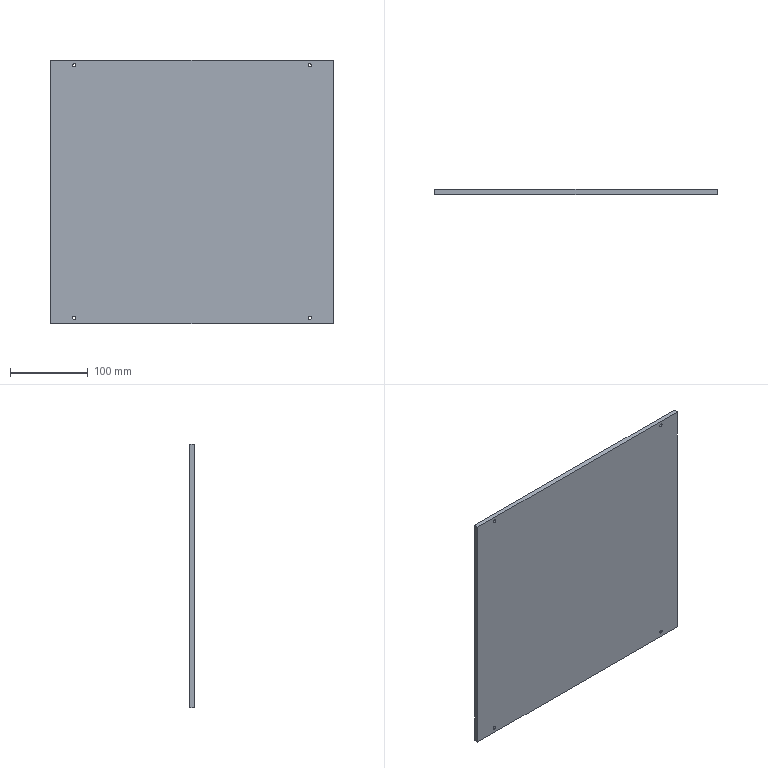Part | SolidWorks | features BaseBody 1 | 1 solid | 30 faces | box 362 x 6 x 337.5 mm | volume 732487 mm3 | cylinder 12 | cone 12 | plane 6 | commonest cylinder face diameters 4.2 x12
STEP:
#1=CARTESIAN_POINT('',(-886.231,800.297,309.232));
#2=VERTEX_POINT('',#1);
#3=CARTESIAN_POINT('',(-884.131,800.297,307.132));
#4=VERTEX_POINT('',#3);
#5=CARTESIAN_POINT('',(-884.131,800.297,309.232));
#6=DIRECTION('',(0.,-1.,0.));
#7=DIRECTION('',(0.,0.,-1.));
#8=AXIS2_PLACEMENT_3D('',#5,#6,#7);
#9=CIRCLE('',#8,2.1);
#10=EDGE_CURVE('',#2,#4,#9,.T.);
#11=ORIENTED_EDGE('',*,*,#10,.T.);
#12=CARTESIAN_POINT('',(-884.131,803.797,307.132));
#13=VERTEX_POINT('',#12);
#14=CARTESIAN_POINT('',(-884.131,806.297,307.132));
#15=DIRECTION('',(0.,1.,0.));
#16=VECTOR('',#15,1000.);
#17=LINE('',#14,#16);
#18=EDGE_CURVE('',#4,#13,#17,.T.);
#19=ORIENTED_EDGE('',*,*,#18,.T.);
#20=CARTESIAN_POINT('',(-886.231,803.797,309.232));
#21=VERTEX_POINT('',#20);
#22=CARTESIAN_POINT('',(-884.131,803.797,309.232));
#23=DIRECTION('',(0.,1.,0.));
#24=DIRECTION('',(1.,0.,-0.000000005));
#25=AXIS2_PLACEMENT_3D('',#22,#23,#24);
#26=CIRCLE('',#25,2.1);
#27=EDGE_CURVE('',#13,#21,#26,.T.);
#28=ORIENTED_EDGE('',*,*,#27,.T.);
#29=CARTESIAN_POINT('',(-886.231,803.797,309.232));
#30=DIRECTION('',(0.,-1.,-0.000000001));
#31=VECTOR('',#30,1000.);
#32=LINE('',#29,#31);
#33=EDGE_CURVE('',#21,#2,#32,.T.);
#34=ORIENTED_EDGE('',*,*,#33,.T.);
#35=EDGE_LOOP('',(#11,#19,#28,#34));
#36=FACE_OUTER_BOUND('',#35,.T.);
#37=CARTESIAN_POINT('',(-884.131,806.297,309.232));
#38=DIRECTION('',(0.,1.,0.));
#39=DIRECTION('',(0.,0.,-1.));
#40=AXIS2_PLACEMENT_3D('',#37,#38,#39);
#41=CYLINDRICAL_SURFACE('',#40,2.1);
#42=ADVANCED_FACE('',(#36),#41,.F.);
#43=ORIENTED_EDGE('',*,*,#27,.F.);
#44=CARTESIAN_POINT('',(-884.131,806.297,304.632));
#45=VERTEX_POINT('',#44);
#46=CARTESIAN_POINT('',(-884.131,805.047,305.882));
#47=DIRECTION('',(0.,0.7071,-0.7071));
#48=VECTOR('',#47,1000.);
#49=LINE('',#46,#48);
#50=EDGE_CURVE('',#13,#45,#49,.T.);
#51=ORIENTED_EDGE('',*,*,#50,.T.);
#52=CARTESIAN_POINT('',(-888.731,806.297,309.232));
#53=VERTEX_POINT('',#52);
#54=CARTESIAN_POINT('',(-884.131,806.297,309.232));
#55=DIRECTION('',(0.,1.,0.));
#56=DIRECTION('',(1.,0.,0.));
#57=AXIS2_PLACEMENT_3D('',#54,#55,#56);
#58=CIRCLE('',#57,4.6);
#59=EDGE_CURVE('',#45,#53,#58,.T.);
#60=ORIENTED_EDGE('',*,*,#59,.T.);
#61=CARTESIAN_POINT('',(-886.231,803.797,309.232));
#62=DIRECTION('',(-0.7071,0.7071,0.000000002));
#63=VECTOR('',#62,1000.);
#64=LINE('',#61,#63);
#65=EDGE_CURVE('',#21,#53,#64,.T.);
#66=ORIENTED_EDGE('',*,*,#65,.F.);
#67=EDGE_LOOP('',(#43,#51,#60,#66));
#68=FACE_OUTER_BOUND('',#67,.T.);
#69=CARTESIAN_POINT('',(-884.131,805.047,309.232));
#70=DIRECTION('',(0.,1.,0.));
#71=DIRECTION('',(0.,0.,-1.));
#72=AXIS2_PLACEMENT_3D('',#69,#70,#71);
#73=CONICAL_SURFACE('',#72,3.35,0.7854);
#74=ADVANCED_FACE('',(#68),#73,.F.);
#75=CARTESIAN_POINT('',(-584.231,800.297,633.232));
#76=VERTEX_POINT('',#75);
#77=CARTESIAN_POINT('',(-582.131,800.297,631.132));
#78=VERTEX_POINT('',#77);
#79=CARTESIAN_POINT('',(-582.131,800.297,633.232));
#80=DIRECTION('',(0.,-1.,0.));
#81=DIRECTION('',(0.,0.,-1.));
#82=AXIS2_PLACEMENT_3D('',#79,#80,#81);
#83=CIRCLE('',#82,2.1);
#84=EDGE_CURVE('',#76,#78,#83,.T.);
#85=ORIENTED_EDGE('',*,*,#84,.T.);
#86=CARTESIAN_POINT('',(-582.131,803.797,631.132));
#87=VERTEX_POINT('',#86);
#88=CARTESIAN_POINT('',(-582.131,806.297,631.132));
#89=DIRECTION('',(0.,1.,0.));
#90=VECTOR('',#89,1000.);
#91=LINE('',#88,#90);
#92=EDGE_CURVE('',#78,#87,#91,.T.);
#93=ORIENTED_EDGE('',*,*,#92,.T.);
#94=CARTESIAN_POINT('',(-584.231,803.797,633.232));
#95=VERTEX_POINT('',#94);
#96=CARTESIAN_POINT('',(-582.131,803.797,633.232));
#97=DIRECTION('',(0.,1.,0.));
#98=DIRECTION('',(1.,0.,-0.000000005));
#99=AXIS2_PLACEMENT_3D('',#96,#97,#98);
#100=CIRCLE('',#99,2.1);
#101=EDGE_CURVE('',#87,#95,#100,.T.);
#102=ORIENTED_EDGE('',*,*,#101,.T.);
#103=CARTESIAN_POINT('',(-584.231,800.297,633.232));
#104=DIRECTION('',(0.,1.,0.000000001));
#105=VECTOR('',#104,1000.);
#106=LINE('',#103,#105);
#107=EDGE_CURVE('',#76,#95,#106,.T.);
#108=ORIENTED_EDGE('',*,*,#107,.F.);
#109=EDGE_LOOP('',(#85,#93,#102,#108));
#110=FACE_OUTER_BOUND('',#109,.T.);
#111=CARTESIAN_POINT('',(-582.131,806.297,633.232));
#112=DIRECTION('',(0.,1.,0.));
#113=DIRECTION('',(0.,0.,-1.));
#114=AXIS2_PLACEMENT_3D('',#111,#112,#113);
#115=CYLINDRICAL_SURFACE('',#114,2.1);
#116=ADVANCED_FACE('',(#110),#115,.F.);
#117=ORIENTED_EDGE('',*,*,#101,.F.);
#118=CARTESIAN_POINT('',(-582.131,806.297,628.632));
#119=VERTEX_POINT('',#118);
#120=CARTESIAN_POINT('',(-582.131,805.047,629.882));
#121=DIRECTION('',(0.,0.7071,-0.7071));
#122=VECTOR('',#121,1000.);
#123=LINE('',#120,#122);
#124=EDGE_CURVE('',#87,#119,#123,.T.);
#125=ORIENTED_EDGE('',*,*,#124,.T.);
#126=CARTESIAN_POINT('',(-586.731,806.297,633.232));
#127=VERTEX_POINT('',#126);
#128=CARTESIAN_POINT('',(-582.131,806.297,633.232));
#129=DIRECTION('',(0.,1.,0.));
#130=DIRECTION('',(0.,0.,-1.));
#131=AXIS2_PLACEMENT_3D('',#128,#129,#130);
#132=CIRCLE('',#131,4.6);
#133=EDGE_CURVE('',#119,#127,#132,.T.);
#134=ORIENTED_EDGE('',*,*,#133,.T.);
#135=CARTESIAN_POINT('',(-586.731,806.297,633.232));
#136=DIRECTION('',(0.7071,-0.7071,-0.000000004));
#137=VECTOR('',#136,1000.);
#138=LINE('',#135,#137);
#139=EDGE_CURVE('',#127,#95,#138,.T.);
#140=ORIENTED_EDGE('',*,*,#139,.T.);
#141=EDGE_LOOP('',(#117,#125,#134,#140));
#142=FACE_OUTER_BOUND('',#141,.T.);
#143=CARTESIAN_POINT('',(-582.131,805.047,633.232));
#144=DIRECTION('',(0.,1.,0.));
#145=DIRECTION('',(0.,0.,-1.));
#146=AXIS2_PLACEMENT_3D('',#143,#144,#145);
#147=CONICAL_SURFACE('',#146,3.35,0.7854);
#148=ADVANCED_FACE('',(#142),#147,.F.);
#149=CARTESIAN_POINT('',(-886.231,800.297,633.232));
#150=VERTEX_POINT('',#149);
#151=CARTESIAN_POINT('',(-884.131,800.297,631.132));
#152=VERTEX_POINT('',#151);
#153=CARTESIAN_POINT('',(-884.131,800.297,633.232));
#154=DIRECTION('',(0.,-1.,0.));
#155=DIRECTION('',(0.,0.,-1.));
#156=AXIS2_PLACEMENT_3D('',#153,#154,#155);
#157=CIRCLE('',#156,2.1);
#158=EDGE_CURVE('',#150,#152,#157,.T.);
#159=ORIENTED_EDGE('',*,*,#158,.T.);
#160=CARTESIAN_POINT('',(-884.131,803.797,631.132));
#161=VERTEX_POINT('',#160);
#162=CARTESIAN_POINT('',(-884.131,806.297,631.132));
#163=DIRECTION('',(0.,1.,0.));
#164=VECTOR('',#163,1000.);
#165=LINE('',#162,#164);
#166=EDGE_CURVE('',#152,#161,#165,.T.);
#167=ORIENTED_EDGE('',*,*,#166,.T.);
#168=CARTESIAN_POINT('',(-886.231,803.797,633.232));
#169=VERTEX_POINT('',#168);
#170=CARTESIAN_POINT('',(-884.131,803.797,633.232));
#171=DIRECTION('',(0.,1.,0.));
#172=DIRECTION('',(1.,0.,-0.000000005));
#173=AXIS2_PLACEMENT_3D('',#170,#171,#172);
#174=CIRCLE('',#173,2.1);
#175=EDGE_CURVE('',#161,#169,#174,.T.);
#176=ORIENTED_EDGE('',*,*,#175,.T.);
#177=CARTESIAN_POINT('',(-886.231,800.297,633.232));
#178=DIRECTION('',(0.,1.,0.000000001));
#179=VECTOR('',#178,1000.);
#180=LINE('',#177,#179);
#181=EDGE_CURVE('',#150,#169,#180,.T.);
#182=ORIENTED_EDGE('',*,*,#181,.F.);
#183=EDGE_LOOP('',(#159,#167,#176,#182));
#184=FACE_OUTER_BOUND('',#183,.T.);
#185=CARTESIAN_POINT('',(-884.131,806.297,633.232));
#186=DIRECTION('',(0.,1.,0.));
#187=DIRECTION('',(0.,0.,-1.));
#188=AXIS2_PLACEMENT_3D('',#185,#186,#187);
#189=CYLINDRICAL_SURFACE('',#188,2.1);
#190=ADVANCED_FACE('',(#184),#189,.F.);
#191=ORIENTED_EDGE('',*,*,#175,.F.);
#192=CARTESIAN_POINT('',(-884.131,806.297,628.632));
#193=VERTEX_POINT('',#192);
#194=CARTESIAN_POINT('',(-884.131,805.047,629.882));
#195=DIRECTION('',(0.,0.7071,-0.7071));
#196=VECTOR('',#195,1000.);
#197=LINE('',#194,#196);
#198=EDGE_CURVE('',#161,#193,#197,.T.);
#199=ORIENTED_EDGE('',*,*,#198,.T.);
#200=CARTESIAN_POINT('',(-888.731,806.297,633.232));
#201=VERTEX_POINT('',#200);
#202=CARTESIAN_POINT('',(-884.131,806.297,633.232));
#203=DIRECTION('',(0.,1.,0.));
#204=DIRECTION('',(0.,0.,-1.));
#205=AXIS2_PLACEMENT_3D('',#202,#203,#204);
#206=CIRCLE('',#205,4.6);
#207=EDGE_CURVE('',#193,#201,#206,.T.);
#208=ORIENTED_EDGE('',*,*,#207,.T.);
#209=CARTESIAN_POINT('',(-888.731,806.297,633.232));
#210=DIRECTION('',(0.7071,-0.7071,-0.000000002));
#211=VECTOR('',#210,1000.);
#212=LINE('',#209,#211);
#213=EDGE_CURVE('',#201,#169,#212,.T.);
#214=ORIENTED_EDGE('',*,*,#213,.T.);
#215=EDGE_LOOP('',(#191,#199,#208,#214));
#216=FACE_OUTER_BOUND('',#215,.T.);
#217=CARTESIAN_POINT('',(-884.131,805.047,633.232));
#218=DIRECTION('',(0.,1.,0.));
#219=DIRECTION('',(0.,0.,-1.));
#220=AXIS2_PLACEMENT_3D('',#217,#218,#219);
#221=CONICAL_SURFACE('',#220,3.35,0.7854);
#222=ADVANCED_FACE('',(#216),#221,.F.);
#223=CARTESIAN_POINT('',(-584.231,800.297,309.232));
#224=VERTEX_POINT('',#223);
#225=CARTESIAN_POINT('',(-582.131,800.297,307.132));
#226=VERTEX_POINT('',#225);
#227=CARTESIAN_POINT('',(-582.131,800.297,309.232));
#228=DIRECTION('',(0.,-1.,0.));
#229=DIRECTION('',(0.,0.,-1.));
#230=AXIS2_PLACEMENT_3D('',#227,#228,#229);
#231=CIRCLE('',#230,2.1);
#232=EDGE_CURVE('',#224,#226,#231,.T.);
#233=ORIENTED_EDGE('',*,*,#232,.T.);
#234=CARTESIAN_POINT('',(-582.131,803.797,307.132));
#235=VERTEX_POINT('',#234);
#236=CARTESIAN_POINT('',(-582.131,806.297,307.132));
#237=DIRECTION('',(0.,1.,0.));
#238=VECTOR('',#237,1000.);
#239=LINE('',#236,#238);
#240=EDGE_CURVE('',#226,#235,#239,.T.);
#241=ORIENTED_EDGE('',*,*,#240,.T.);
#242=CARTESIAN_POINT('',(-584.231,803.797,309.232));
#243=VERTEX_POINT('',#242);
#244=CARTESIAN_POINT('',(-582.131,803.797,309.232));
#245=DIRECTION('',(0.,1.,0.));
#246=DIRECTION('',(1.,0.,-0.000000005));
#247=AXIS2_PLACEMENT_3D('',#244,#245,#246);
#248=CIRCLE('',#247,2.1);
#249=EDGE_CURVE('',#235,#243,#248,.T.);
#250=ORIENTED_EDGE('',*,*,#249,.T.);
#251=CARTESIAN_POINT('',(-584.231,803.797,309.232));
#252=DIRECTION('',(0.,-1.,-0.000000001));
#253=VECTOR('',#252,1000.);
#254=LINE('',#251,#253);
#255=EDGE_CURVE('',#243,#224,#254,.T.);
#256=ORIENTED_EDGE('',*,*,#255,.T.);
#257=EDGE_LOOP('',(#233,#241,#250,#256));
#258=FACE_OUTER_BOUND('',#257,.T.);
#259=CARTESIAN_POINT('',(-582.131,806.297,309.232));
#260=DIRECTION('',(0.,1.,0.));
#261=DIRECTION('',(0.,0.,-1.));
#262=AXIS2_PLACEMENT_3D('',#259,#260,#261);
#263=CYLINDRICAL_SURFACE('',#262,2.1);
#264=ADVANCED_FACE('',(#258),#263,.F.);
#265=ORIENTED_EDGE('',*,*,#249,.F.);
#266=CARTESIAN_POINT('',(-582.131,806.297,304.632));
#267=VERTEX_POINT('',#266);
#268=CARTESIAN_POINT('',(-582.131,805.047,305.882));
#269=DIRECTION('',(0.,0.7071,-0.7071));
#270=VECTOR('',#269,1000.);
#271=LINE('',#268,#270);
#272=EDGE_CURVE('',#235,#267,#271,.T.);
#273=ORIENTED_EDGE('',*,*,#272,.T.);
#274=CARTESIAN_POINT('',(-586.731,806.297,309.232));
#275=VERTEX_POINT('',#274);
#276=CARTESIAN_POINT('',(-582.131,806.297,309.232));
#277=DIRECTION('',(0.,1.,0.));
#278=DIRECTION('',(1.,0.,-0.000000003));
#279=AXIS2_PLACEMENT_3D('',#276,#277,#278);
#280=CIRCLE('',#279,4.6);
#281=EDGE_CURVE('',#267,#275,#280,.T.);
#282=ORIENTED_EDGE('',*,*,#281,.T.);
#283=CARTESIAN_POINT('',(-586.731,806.297,309.232));
#284=DIRECTION('',(0.7071,-0.7071,-0.000000002));
#285=VECTOR('',#284,1000.);
#286=LINE('',#283,#285);
#287=EDGE_CURVE('',#275,#243,#286,.T.);
#288=ORIENTED_EDGE('',*,*,#287,.T.);
#289=EDGE_LOOP('',(#265,#273,#282,#288));
#290=FACE_OUTER_BOUND('',#289,.T.);
#291=CARTESIAN_POINT('',(-582.131,805.047,309.232));
#292=DIRECTION('',(0.,1.,0.));
#293=DIRECTION('',(0.,0.,-1.));
#294=AXIS2_PLACEMENT_3D('',#291,#292,#293);
#295=CONICAL_SURFACE('',#294,3.35,0.7854);
#296=ADVANCED_FACE('',(#290),#295,.F.);
#297=CARTESIAN_POINT('',(-552.131,800.297,301.732));
#298=VERTEX_POINT('',#297);
#299=CARTESIAN_POINT('',(-914.131,800.297,301.732));
#300=VERTEX_POINT('',#299);
#301=CARTESIAN_POINT('',(-552.131,800.297,301.732));
#302=DIRECTION('',(-1.,0.,0.));
#303=VECTOR('',#302,1000.);
#304=LINE('',#301,#303);
#305=EDGE_CURVE('',#298,#300,#304,.T.);
#306=ORIENTED_EDGE('',*,*,#305,.F.);
#307=CARTESIAN_POINT('',(-552.131,800.297,639.232));
#308=VERTEX_POINT('',#307);
#309=CARTESIAN_POINT('',(-552.131,800.297,639.232));
#310=DIRECTION('',(0.,0.,-1.));
#311=VECTOR('',#310,1000.);
#312=LINE('',#309,#311);
#313=EDGE_CURVE('',#308,#298,#312,.T.);
#314=ORIENTED_EDGE('',*,*,#313,.F.);
#315=CARTESIAN_POINT('',(-914.131,800.297,639.232));
#316=VERTEX_POINT('',#315);
#317=CARTESIAN_POINT('',(-914.131,800.297,639.232));
#318=DIRECTION('',(1.,0.,0.));
#319=VECTOR('',#318,1000.);
#320=LINE('',#317,#319);
#321=EDGE_CURVE('',#316,#308,#320,.T.);
#322=ORIENTED_EDGE('',*,*,#321,.F.);
#323=CARTESIAN_POINT('',(-914.131,800.297,301.732));
#324=DIRECTION('',(0.,0.,1.));
#325=VECTOR('',#324,1000.);
#326=LINE('',#323,#325);
#327=EDGE_CURVE('',#300,#316,#326,.T.);
#328=ORIENTED_EDGE('',*,*,#327,.F.);
#329=EDGE_LOOP('',(#306,#314,#322,#328));
#330=FACE_OUTER_BOUND('',#329,.T.);
#331=ORIENTED_EDGE('',*,*,#10,.F.);
#332=CARTESIAN_POINT('',(-882.031,800.297,309.232));
#333=VERTEX_POINT('',#332);
#334=CARTESIAN_POINT('',(-884.131,800.297,309.232));
#335=DIRECTION('',(0.,-1.,0.));
#336=DIRECTION('',(1.,0.,0.));
#337=AXIS2_PLACEMENT_3D('',#334,#335,#336);
#338=CIRCLE('',#337,2.1);
#339=EDGE_CURVE('',#333,#2,#338,.T.);
#340=ORIENTED_EDGE('',*,*,#339,.F.);
#341=CARTESIAN_POINT('',(-884.131,800.297,309.232));
#342=DIRECTION('',(0.,-1.,0.));
#343=DIRECTION('',(0.,0.,-1.));
#344=AXIS2_PLACEMENT_3D('',#341,#342,#343);
#345=CIRCLE('',#344,2.1);
#346=EDGE_CURVE('',#4,#333,#345,.T.);
#347=ORIENTED_EDGE('',*,*,#346,.F.);
#348=EDGE_LOOP('',(#331,#340,#347));
#349=FACE_BOUND('',#348,.T.);
#350=ORIENTED_EDGE('',*,*,#84,.F.);
#351=CARTESIAN_POINT('',(-580.031,800.297,633.232));
#352=VERTEX_POINT('',#351);
#353=CARTESIAN_POINT('',(-582.131,800.297,633.232));
#354=DIRECTION('',(0.,-1.,0.));
#355=DIRECTION('',(1.,0.,0.));
#356=AXIS2_PLACEMENT_3D('',#353,#354,#355);
#357=CIRCLE('',#356,2.1);
#358=EDGE_CURVE('',#352,#76,#357,.T.);
#359=ORIENTED_EDGE('',*,*,#358,.F.);
#360=CARTESIAN_POINT('',(-582.131,800.297,633.232));
#361=DIRECTION('',(0.,-1.,0.));
#362=DIRECTION('',(0.,0.,-1.));
#363=AXIS2_PLACEMENT_3D('',#360,#361,#362);
#364=CIRCLE('',#363,2.1);
#365=EDGE_CURVE('',#78,#352,#364,.T.);
#366=ORIENTED_EDGE('',*,*,#365,.F.);
#367=EDGE_LOOP('',(#350,#359,#366));
#368=FACE_BOUND('',#367,.T.);
#369=ORIENTED_EDGE('',*,*,#158,.F.);
#370=CARTESIAN_POINT('',(-882.031,800.297,633.232));
#371=VERTEX_POINT('',#370);
#372=CARTESIAN_POINT('',(-884.131,800.297,633.232));
#373=DIRECTION('',(0.,-1.,0.));
#374=DIRECTION('',(1.,0.,0.));
#375=AXIS2_PLACEMENT_3D('',#372,#373,#374);
#376=CIRCLE('',#375,2.1);
#377=EDGE_CURVE('',#371,#150,#376,.T.);
#378=ORIENTED_EDGE('',*,*,#377,.F.);
#379=CARTESIAN_POINT('',(-884.131,800.297,633.232));
#380=DIRECTION('',(0.,-1.,0.));
#381=DIRECTION('',(0.,0.,-1.));
#382=AXIS2_PLACEMENT_3D('',#379,#380,#381);
#383=CIRCLE('',#382,2.1);
#384=EDGE_CURVE('',#152,#371,#383,.T.);
#385=ORIENTED_EDGE('',*,*,#384,.F.);
#386=EDGE_LOOP('',(#369,#378,#385));
#387=FACE_BOUND('',#386,.T.);
#388=ORIENTED_EDGE('',*,*,#232,.F.);
#389=CARTESIAN_POINT('',(-580.031,800.297,309.232));
#390=VERTEX_POINT('',#389);
#391=CARTESIAN_POINT('',(-582.131,800.297,309.232));
#392=DIRECTION('',(0.,-1.,0.));
#393=DIRECTION('',(1.,0.,0.));
#394=AXIS2_PLACEMENT_3D('',#391,#392,#393);
#395=CIRCLE('',#394,2.1);
#396=EDGE_CURVE('',#390,#224,#395,.T.);
#397=ORIENTED_EDGE('',*,*,#396,.F.);
#398=CARTESIAN_POINT('',(-582.131,800.297,309.232));
#399=DIRECTION('',(0.,-1.,0.));
#400=DIRECTION('',(0.,0.,-1.));
#401=AXIS2_PLACEMENT_3D('',#398,#399,#400);
#402=CIRCLE('',#401,2.1);
#403=EDGE_CURVE('',#226,#390,#402,.T.);
#404=ORIENTED_EDGE('',*,*,#403,.F.);
#405=EDGE_LOOP('',(#388,#397,#404));
#406=FACE_BOUND('',#405,.T.);
#407=CARTESIAN_POINT('',(-936.11,800.297,658.732));
#408=DIRECTION('',(0.,-1.,0.));
#409=DIRECTION('',(-1.,0.,0.));
#410=AXIS2_PLACEMENT_3D('',#407,#408,#409);
#411=PLANE('',#410);
#412=ADVANCED_FACE('',(#330,#349,#368,#387,#406),#411,.T.);
#413=CARTESIAN_POINT('',(-914.131,806.297,301.732));
#414=VERTEX_POINT('',#413);
#415=CARTESIAN_POINT('',(-914.131,800.297,301.732));
#416=DIRECTION('',(0.,1.,0.));
#417=VECTOR('',#416,1000.);
#418=LINE('',#415,#417);
#419=EDGE_CURVE('',#300,#414,#418,.T.);
#420=ORIENTED_EDGE('',*,*,#419,.F.);
#421=ORIENTED_EDGE('',*,*,#327,.T.);
#422=CARTESIAN_POINT('',(-914.131,806.297,639.232));
#423=VERTEX_POINT('',#422);
#424=CARTESIAN_POINT('',(-914.131,800.297,639.232));
#425=DIRECTION('',(0.,1.,0.));
#426=VECTOR('',#425,1000.);
#427=LINE('',#424,#426);
#428=EDGE_CURVE('',#316,#423,#427,.T.);
#429=ORIENTED_EDGE('',*,*,#428,.T.);
#430=CARTESIAN_POINT('',(-914.131,806.297,639.232));
#431=DIRECTION('',(0.,0.,-1.));
#432=VECTOR('',#431,1000.);
#433=LINE('',#430,#432);
#434=EDGE_CURVE('',#423,#414,#433,.T.);
#435=ORIENTED_EDGE('',*,*,#434,.T.);
#436=EDGE_LOOP('',(#420,#421,#429,#435));
#437=FACE_OUTER_BOUND('',#436,.T.);
#438=CARTESIAN_POINT('',(-914.131,806.297,301.732));
#439=DIRECTION('',(-1.,0.,0.));
#440=DIRECTION('',(0.,0.,-1.));
#441=AXIS2_PLACEMENT_3D('',#438,#439,#440);
#442=PLANE('',#441);
#443=ADVANCED_FACE('',(#437),#442,.T.);
#444=CARTESIAN_POINT('',(-552.131,806.297,301.732));
#445=VERTEX_POINT('',#444);
#446=CARTESIAN_POINT('',(-914.131,806.297,301.732));
#447=DIRECTION('',(1.,0.,0.));
#448=VECTOR('',#447,1000.);
#449=LINE('',#446,#448);
#450=EDGE_CURVE('',#414,#445,#449,.T.);
#451=ORIENTED_EDGE('',*,*,#450,.F.);
#452=ORIENTED_EDGE('',*,*,#434,.F.);
#453=CARTESIAN_POINT('',(-552.131,806.297,639.232));
#454=VERTEX_POINT('',#453);
#455=CARTESIAN_POINT('',(-552.131,806.297,639.232));
#456=DIRECTION('',(-1.,0.,0.));
#457=VECTOR('',#456,1000.);
#458=LINE('',#455,#457);
#459=EDGE_CURVE('',#454,#423,#458,.T.);
#460=ORIENTED_EDGE('',*,*,#459,.F.);
#461=CARTESIAN_POINT('',(-552.131,806.297,301.732));
#462=DIRECTION('',(0.,0.,1.));
#463=VECTOR('',#462,1000.);
#464=LINE('',#461,#463);
#465=EDGE_CURVE('',#445,#454,#464,.T.);
#466=ORIENTED_EDGE('',*,*,#465,.F.);
#467=EDGE_LOOP('',(#451,#452,#460,#466));
#468=FACE_OUTER_BOUND('',#467,.T.);
#469=CARTESIAN_POINT('',(-577.531,806.297,309.232));
#470=VERTEX_POINT('',#469);
#471=CARTESIAN_POINT('',(-582.131,806.297,309.232));
#472=DIRECTION('',(0.,1.,0.));
#473=DIRECTION('',(0.,0.,1.));
#474=AXIS2_PLACEMENT_3D('',#471,#472,#473);
#475=CIRCLE('',#474,4.6);
#476=EDGE_CURVE('',#275,#470,#475,.T.);
#477=ORIENTED_EDGE('',*,*,#476,.F.);
#478=ORIENTED_EDGE('',*,*,#281,.F.);
#479=CARTESIAN_POINT('',(-582.131,806.297,309.232));
#480=DIRECTION('',(0.,1.,0.));
#481=DIRECTION('',(1.,0.,-0.000000003));
#482=AXIS2_PLACEMENT_3D('',#479,#480,#481);
#483=CIRCLE('',#482,4.6);
#484=EDGE_CURVE('',#470,#267,#483,.T.);
#485=ORIENTED_EDGE('',*,*,#484,.F.);
#486=EDGE_LOOP('',(#477,#478,#485));
#487=FACE_BOUND('',#486,.T.);
#488=CARTESIAN_POINT('',(-879.531,806.297,633.232));
#489=VERTEX_POINT('',#488);
#490=CARTESIAN_POINT('',(-884.131,806.297,633.232));
#491=DIRECTION('',(0.,1.,0.));
#492=DIRECTION('',(0.,0.,-1.));
#493=AXIS2_PLACEMENT_3D('',#490,#491,#492);
#494=CIRCLE('',#493,4.6);
#495=EDGE_CURVE('',#489,#193,#494,.T.);
#496=ORIENTED_EDGE('',*,*,#495,.F.);
#497=CARTESIAN_POINT('',(-884.131,806.297,633.232));
#498=DIRECTION('',(0.,1.,0.));
#499=DIRECTION('',(-1.,0.,0.));
#500=AXIS2_PLACEMENT_3D('',#497,#498,#499);
#501=CIRCLE('',#500,4.6);
#502=EDGE_CURVE('',#201,#489,#501,.T.);
#503=ORIENTED_EDGE('',*,*,#502,.F.);
#504=ORIENTED_EDGE('',*,*,#207,.F.);
#505=EDGE_LOOP('',(#496,#503,#504));
#506=FACE_BOUND('',#505,.T.);
#507=CARTESIAN_POINT('',(-577.531,806.297,633.232));
#508=VERTEX_POINT('',#507);
#509=CARTESIAN_POINT('',(-582.131,806.297,633.232));
#510=DIRECTION('',(0.,1.,0.));
#511=DIRECTION('',(0.,0.,-1.));
#512=AXIS2_PLACEMENT_3D('',#509,#510,#511);
#513=CIRCLE('',#512,4.6);
#514=EDGE_CURVE('',#508,#119,#513,.T.);
#515=ORIENTED_EDGE('',*,*,#514,.F.);
#516=CARTESIAN_POINT('',(-582.131,806.297,633.232));
#517=DIRECTION('',(0.,1.,0.));
#518=DIRECTION('',(-1.,0.,0.000000003));
#519=AXIS2_PLACEMENT_3D('',#516,#517,#518);
#520=CIRCLE('',#519,4.6);
#521=EDGE_CURVE('',#127,#508,#520,.T.);
#522=ORIENTED_EDGE('',*,*,#521,.F.);
#523=ORIENTED_EDGE('',*,*,#133,.F.);
#524=EDGE_LOOP('',(#515,#522,#523));
#525=FACE_BOUND('',#524,.T.);
#526=CARTESIAN_POINT('',(-879.531,806.297,309.232));
#527=VERTEX_POINT('',#526);
#528=CARTESIAN_POINT('',(-884.131,806.297,309.232));
#529=DIRECTION('',(0.,1.,0.));
#530=DIRECTION('',(0.,0.,1.));
#531=AXIS2_PLACEMENT_3D('',#528,#529,#530);
#532=CIRCLE('',#531,4.6);
#533=EDGE_CURVE('',#53,#527,#532,.T.);
#534=ORIENTED_EDGE('',*,*,#533,.F.);
#535=ORIENTED_EDGE('',*,*,#59,.F.);
#536=CARTESIAN_POINT('',(-884.131,806.297,309.232));
#537=DIRECTION('',(0.,1.,0.));
#538=DIRECTION('',(1.,0.,0.));
#539=AXIS2_PLACEMENT_3D('',#536,#537,#538);
#540=CIRCLE('',#539,4.6);
#541=EDGE_CURVE('',#527,#45,#540,.T.);
#542=ORIENTED_EDGE('',*,*,#541,.F.);
#543=EDGE_LOOP('',(#534,#535,#542));
#544=FACE_BOUND('',#543,.T.);
#545=CARTESIAN_POINT('',(-524.111,806.297,658.732));
#546=DIRECTION('',(0.,1.,0.));
#547=DIRECTION('',(1.,0.,0.));
#548=AXIS2_PLACEMENT_3D('',#545,#546,#547);
#549=PLANE('',#548);
#550=ADVANCED_FACE('',(#468,#487,#506,#525,#544),#549,.T.);
#551=CARTESIAN_POINT('',(-552.131,800.297,301.732));
#552=DIRECTION('',(0.,1.,0.));
#553=VECTOR('',#552,1000.);
#554=LINE('',#551,#553);
#555=EDGE_CURVE('',#298,#445,#554,.T.);
#556=ORIENTED_EDGE('',*,*,#555,.T.);
#557=ORIENTED_EDGE('',*,*,#465,.T.);
#558=CARTESIAN_POINT('',(-552.131,806.297,639.232));
#559=DIRECTION('',(0.,-1.,0.));
#560=VECTOR('',#559,1000.);
#561=LINE('',#558,#560);
#562=EDGE_CURVE('',#454,#308,#561,.T.);
#563=ORIENTED_EDGE('',*,*,#562,.T.);
#564=ORIENTED_EDGE('',*,*,#313,.T.);
#565=EDGE_LOOP('',(#556,#557,#563,#564));
#566=FACE_OUTER_BOUND('',#565,.T.);
#567=CARTESIAN_POINT('',(-552.131,806.297,658.732));
#568=DIRECTION('',(1.,0.,0.));
#569=DIRECTION('',(0.,0.,1.));
#570=AXIS2_PLACEMENT_3D('',#567,#568,#569);
#571=PLANE('',#570);
#572=ADVANCED_FACE('',(#566),#571,.T.);
#573=ORIENTED_EDGE('',*,*,#459,.T.);
#574=ORIENTED_EDGE('',*,*,#428,.F.);
#575=ORIENTED_EDGE('',*,*,#321,.T.);
#576=ORIENTED_EDGE('',*,*,#562,.F.);
#577=EDGE_LOOP('',(#573,#574,#575,#576));
#578=FACE_OUTER_BOUND('',#577,.T.);
#579=CARTESIAN_POINT('',(-552.131,806.297,639.232));
#580=DIRECTION('',(0.,0.,-1.));
#581=DIRECTION('',(1.,0.,0.));
#582=AXIS2_PLACEMENT_3D('',#579,#580,#581);
#583=PLANE('',#582);
#584=ADVANCED_FACE('',(#578),#583,.F.);
#585=ORIENTED_EDGE('',*,*,#305,.T.);
#586=ORIENTED_EDGE('',*,*,#419,.T.);
#587=ORIENTED_EDGE('',*,*,#450,.T.);
#588=ORIENTED_EDGE('',*,*,#555,.F.);
#589=EDGE_LOOP('',(#585,#586,#587,#588));
#590=FACE_OUTER_BOUND('',#589,.T.);
#591=CARTESIAN_POINT('',(-524.111,806.297,301.732));
#592=DIRECTION('',(0.,0.,-1.));
#593=DIRECTION('',(1.,0.,0.));
#594=AXIS2_PLACEMENT_3D('',#591,#592,#593);
#595=PLANE('',#594);
#596=ADVANCED_FACE('',(#590),#595,.T.);
#597=CARTESIAN_POINT('',(-580.031,803.797,309.232));
#598=VERTEX_POINT('',#597);
#599=CARTESIAN_POINT('',(-580.031,803.797,309.232));
#600=DIRECTION('',(0.7071,0.7071,-0.000000004));
#601=VECTOR('',#600,1000.);
#602=LINE('',#599,#601);
#603=EDGE_CURVE('',#598,#470,#602,.T.);
#604=ORIENTED_EDGE('',*,*,#603,.F.);
#605=CARTESIAN_POINT('',(-582.131,803.797,309.232));
#606=DIRECTION('',(0.,1.,0.));
#607=DIRECTION('',(-1.,0.,0.000000005));
#608=AXIS2_PLACEMENT_3D('',#605,#606,#607);
#609=CIRCLE('',#608,2.1);
#610=EDGE_CURVE('',#243,#598,#609,.T.);
#611=ORIENTED_EDGE('',*,*,#610,.F.);
#612=ORIENTED_EDGE('',*,*,#287,.F.);
#613=ORIENTED_EDGE('',*,*,#476,.T.);
#614=EDGE_LOOP('',(#604,#611,#612,#613));
#615=FACE_OUTER_BOUND('',#614,.T.);
#616=CARTESIAN_POINT('',(-582.131,805.047,309.232));
#617=DIRECTION('',(0.,1.,0.));
#618=DIRECTION('',(0.,0.,-1.));
#619=AXIS2_PLACEMENT_3D('',#616,#617,#618);
#620=CONICAL_SURFACE('',#619,3.35,0.7854);
#621=ADVANCED_FACE('',(#615),#620,.F.);
#622=ORIENTED_EDGE('',*,*,#272,.F.);
#623=CARTESIAN_POINT('',(-582.131,803.797,309.232));
#624=DIRECTION('',(0.,1.,0.));
#625=DIRECTION('',(1.,0.,-0.000000005));
#626=AXIS2_PLACEMENT_3D('',#623,#624,#625);
#627=CIRCLE('',#626,2.1);
#628=EDGE_CURVE('',#598,#235,#627,.T.);
#629=ORIENTED_EDGE('',*,*,#628,.F.);
#630=ORIENTED_EDGE('',*,*,#603,.T.);
#631=ORIENTED_EDGE('',*,*,#484,.T.);
#632=EDGE_LOOP('',(#622,#629,#630,#631));
#633=FACE_OUTER_BOUND('',#632,.T.);
#634=CARTESIAN_POINT('',(-582.131,805.047,309.232));
#635=DIRECTION('',(0.,1.,0.));
#636=DIRECTION('',(0.,0.,-1.));
#637=AXIS2_PLACEMENT_3D('',#634,#635,#636);
#638=CONICAL_SURFACE('',#637,3.35,0.7854);
#639=ADVANCED_FACE('',(#633),#638,.F.);
#640=ORIENTED_EDGE('',*,*,#240,.F.);
#641=ORIENTED_EDGE('',*,*,#403,.T.);
#642=CARTESIAN_POINT('',(-580.031,800.297,309.232));
#643=DIRECTION('',(0.,1.,-0.000000001));
#644=VECTOR('',#643,1000.);
#645=LINE('',#642,#644);
#646=EDGE_CURVE('',#390,#598,#645,.T.);
#647=ORIENTED_EDGE('',*,*,#646,.T.);
#648=ORIENTED_EDGE('',*,*,#628,.T.);
#649=EDGE_LOOP('',(#640,#641,#647,#648));
#650=FACE_OUTER_BOUND('',#649,.T.);
#651=CARTESIAN_POINT('',(-582.131,806.297,309.232));
#652=DIRECTION('',(0.,1.,0.));
#653=DIRECTION('',(0.,0.,-1.));
#654=AXIS2_PLACEMENT_3D('',#651,#652,#653);
#655=CYLINDRICAL_SURFACE('',#654,2.1);
#656=ADVANCED_FACE('',(#650),#655,.F.);
#657=ORIENTED_EDGE('',*,*,#396,.T.);
#658=ORIENTED_EDGE('',*,*,#255,.F.);
#659=ORIENTED_EDGE('',*,*,#610,.T.);
#660=ORIENTED_EDGE('',*,*,#646,.F.);
#661=EDGE_LOOP('',(#657,#658,#659,#660));
#662=FACE_OUTER_BOUND('',#661,.T.);
#663=CARTESIAN_POINT('',(-582.131,806.297,309.232));
#664=DIRECTION('',(0.,1.,0.));
#665=DIRECTION('',(0.,0.,-1.));
#666=AXIS2_PLACEMENT_3D('',#663,#664,#665);
#667=CYLINDRICAL_SURFACE('',#666,2.1);
#668=ADVANCED_FACE('',(#662),#667,.F.);
#669=ORIENTED_EDGE('',*,*,#198,.F.);
#670=CARTESIAN_POINT('',(-882.031,803.797,633.232));
#671=VERTEX_POINT('',#670);
#672=CARTESIAN_POINT('',(-884.131,803.797,633.232));
#673=DIRECTION('',(0.,1.,0.));
#674=DIRECTION('',(1.,0.,-0.000000005));
#675=AXIS2_PLACEMENT_3D('',#672,#673,#674);
#676=CIRCLE('',#675,2.1);
#677=EDGE_CURVE('',#671,#161,#676,.T.);
#678=ORIENTED_EDGE('',*,*,#677,.F.);
#679=CARTESIAN_POINT('',(-882.031,803.797,633.232));
#680=DIRECTION('',(0.7071,0.7071,-0.000000004));
#681=VECTOR('',#680,1000.);
#682=LINE('',#679,#681);
#683=EDGE_CURVE('',#671,#489,#682,.T.);
#684=ORIENTED_EDGE('',*,*,#683,.T.);
#685=ORIENTED_EDGE('',*,*,#495,.T.);
#686=EDGE_LOOP('',(#669,#678,#684,#685));
#687=FACE_OUTER_BOUND('',#686,.T.);
#688=CARTESIAN_POINT('',(-884.131,805.047,633.232));
#689=DIRECTION('',(0.,1.,0.));
#690=DIRECTION('',(0.,0.,-1.));
#691=AXIS2_PLACEMENT_3D('',#688,#689,#690);
#692=CONICAL_SURFACE('',#691,3.35,0.7854);
#693=ADVANCED_FACE('',(#687),#692,.F.);
#694=ORIENTED_EDGE('',*,*,#683,.F.);
#695=CARTESIAN_POINT('',(-884.131,803.797,633.232));
#696=DIRECTION('',(0.,1.,0.));
#697=DIRECTION('',(-1.,0.,0.000000005));
#698=AXIS2_PLACEMENT_3D('',#695,#696,#697);
#699=CIRCLE('',#698,2.1);
#700=EDGE_CURVE('',#169,#671,#699,.T.);
#701=ORIENTED_EDGE('',*,*,#700,.F.);
#702=ORIENTED_EDGE('',*,*,#213,.F.);
#703=ORIENTED_EDGE('',*,*,#502,.T.);
#704=EDGE_LOOP('',(#694,#701,#702,#703));
#705=FACE_OUTER_BOUND('',#704,.T.);
#706=CARTESIAN_POINT('',(-884.131,805.047,633.232));
#707=DIRECTION('',(0.,1.,0.));
#708=DIRECTION('',(0.,0.,-1.));
#709=AXIS2_PLACEMENT_3D('',#706,#707,#708);
#710=CONICAL_SURFACE('',#709,3.35,0.7854);
#711=ADVANCED_FACE('',(#705),#710,.F.);
#712=ORIENTED_EDGE('',*,*,#377,.T.);
#713=ORIENTED_EDGE('',*,*,#181,.T.);
#714=ORIENTED_EDGE('',*,*,#700,.T.);
#715=CARTESIAN_POINT('',(-882.031,803.797,633.232));
#716=DIRECTION('',(0.,-1.,0.000000001));
#717=VECTOR('',#716,1000.);
#718=LINE('',#715,#717);
#719=EDGE_CURVE('',#671,#371,#718,.T.);
#720=ORIENTED_EDGE('',*,*,#719,.T.);
#721=EDGE_LOOP('',(#712,#713,#714,#720));
#722=FACE_OUTER_BOUND('',#721,.T.);
#723=CARTESIAN_POINT('',(-884.131,806.297,633.232));
#724=DIRECTION('',(0.,1.,0.));
#725=DIRECTION('',(0.,0.,-1.));
#726=AXIS2_PLACEMENT_3D('',#723,#724,#725);
#727=CYLINDRICAL_SURFACE('',#726,2.1);
#728=ADVANCED_FACE('',(#722),#727,.F.);
#729=ORIENTED_EDGE('',*,*,#166,.F.);
#730=ORIENTED_EDGE('',*,*,#384,.T.);
#731=ORIENTED_EDGE('',*,*,#719,.F.);
#732=ORIENTED_EDGE('',*,*,#677,.T.);
#733=EDGE_LOOP('',(#729,#730,#731,#732));
#734=FACE_OUTER_BOUND('',#733,.T.);
#735=CARTESIAN_POINT('',(-884.131,806.297,633.232));
#736=DIRECTION('',(0.,1.,0.));
#737=DIRECTION('',(0.,0.,-1.));
#738=AXIS2_PLACEMENT_3D('',#735,#736,#737);
#739=CYLINDRICAL_SURFACE('',#738,2.1);
#740=ADVANCED_FACE('',(#734),#739,.F.);
#741=ORIENTED_EDGE('',*,*,#124,.F.);
#742=CARTESIAN_POINT('',(-580.031,803.797,633.232));
#743=VERTEX_POINT('',#742);
#744=CARTESIAN_POINT('',(-582.131,803.797,633.232));
#745=DIRECTION('',(0.,1.,0.));
#746=DIRECTION('',(1.,0.,-0.000000005));
#747=AXIS2_PLACEMENT_3D('',#744,#745,#746);
#748=CIRCLE('',#747,2.1);
#749=EDGE_CURVE('',#743,#87,#748,.T.);
#750=ORIENTED_EDGE('',*,*,#749,.F.);
#751=CARTESIAN_POINT('',(-580.031,803.797,633.232));
#752=DIRECTION('',(0.7071,0.7071,-0.000000004));
#753=VECTOR('',#752,1000.);
#754=LINE('',#751,#753);
#755=EDGE_CURVE('',#743,#508,#754,.T.);
#756=ORIENTED_EDGE('',*,*,#755,.T.);
#757=ORIENTED_EDGE('',*,*,#514,.T.);
#758=EDGE_LOOP('',(#741,#750,#756,#757));
#759=FACE_OUTER_BOUND('',#758,.T.);
#760=CARTESIAN_POINT('',(-582.131,805.047,633.232));
#761=DIRECTION('',(0.,1.,0.));
#762=DIRECTION('',(0.,0.,-1.));
#763=AXIS2_PLACEMENT_3D('',#760,#761,#762);
#764=CONICAL_SURFACE('',#763,3.35,0.7854);
#765=ADVANCED_FACE('',(#759),#764,.F.);
#766=ORIENTED_EDGE('',*,*,#755,.F.);
#767=CARTESIAN_POINT('',(-582.131,803.797,633.232));
#768=DIRECTION('',(0.,1.,0.));
#769=DIRECTION('',(-1.,0.,0.000000005));
#770=AXIS2_PLACEMENT_3D('',#767,#768,#769);
#771=CIRCLE('',#770,2.1);
#772=EDGE_CURVE('',#95,#743,#771,.T.);
#773=ORIENTED_EDGE('',*,*,#772,.F.);
#774=ORIENTED_EDGE('',*,*,#139,.F.);
#775=ORIENTED_EDGE('',*,*,#521,.T.);
#776=EDGE_LOOP('',(#766,#773,#774,#775));
#777=FACE_OUTER_BOUND('',#776,.T.);
#778=CARTESIAN_POINT('',(-582.131,805.047,633.232));
#779=DIRECTION('',(0.,1.,0.));
#780=DIRECTION('',(0.,0.,-1.));
#781=AXIS2_PLACEMENT_3D('',#778,#779,#780);
#782=CONICAL_SURFACE('',#781,3.35,0.7854);
#783=ADVANCED_FACE('',(#777),#782,.F.);
#784=ORIENTED_EDGE('',*,*,#358,.T.);
#785=ORIENTED_EDGE('',*,*,#107,.T.);
#786=ORIENTED_EDGE('',*,*,#772,.T.);
#787=CARTESIAN_POINT('',(-580.031,803.797,633.232));
#788=DIRECTION('',(0.,-1.,0.000000001));
#789=VECTOR('',#788,1000.);
#790=LINE('',#787,#789);
#791=EDGE_CURVE('',#743,#352,#790,.T.);
#792=ORIENTED_EDGE('',*,*,#791,.T.);
#793=EDGE_LOOP('',(#784,#785,#786,#792));
#794=FACE_OUTER_BOUND('',#793,.T.);
#795=CARTESIAN_POINT('',(-582.131,806.297,633.232));
#796=DIRECTION('',(0.,1.,0.));
#797=DIRECTION('',(0.,0.,-1.));
#798=AXIS2_PLACEMENT_3D('',#795,#796,#797);
#799=CYLINDRICAL_SURFACE('',#798,2.1);
#800=ADVANCED_FACE('',(#794),#799,.F.);
#801=ORIENTED_EDGE('',*,*,#92,.F.);
#802=ORIENTED_EDGE('',*,*,#365,.T.);
#803=ORIENTED_EDGE('',*,*,#791,.F.);
#804=ORIENTED_EDGE('',*,*,#749,.T.);
#805=EDGE_LOOP('',(#801,#802,#803,#804));
#806=FACE_OUTER_BOUND('',#805,.T.);
#807=CARTESIAN_POINT('',(-582.131,806.297,633.232));
#808=DIRECTION('',(0.,1.,0.));
#809=DIRECTION('',(0.,0.,-1.));
#810=AXIS2_PLACEMENT_3D('',#807,#808,#809);
#811=CYLINDRICAL_SURFACE('',#810,2.1);
#812=ADVANCED_FACE('',(#806),#811,.F.);
#813=CARTESIAN_POINT('',(-882.031,803.797,309.232));
#814=VERTEX_POINT('',#813);
#815=CARTESIAN_POINT('',(-879.531,806.297,309.232));
#816=DIRECTION('',(-0.7071,-0.7071,0.000000002));
#817=VECTOR('',#816,1000.);
#818=LINE('',#815,#817);
#819=EDGE_CURVE('',#527,#814,#818,.T.);
#820=ORIENTED_EDGE('',*,*,#819,.T.);
#821=CARTESIAN_POINT('',(-884.131,803.797,309.232));
#822=DIRECTION('',(0.,1.,0.));
#823=DIRECTION('',(-1.,0.,0.000000005));
#824=AXIS2_PLACEMENT_3D('',#821,#822,#823);
#825=CIRCLE('',#824,2.1);
#826=EDGE_CURVE('',#21,#814,#825,.T.);
#827=ORIENTED_EDGE('',*,*,#826,.F.);
#828=ORIENTED_EDGE('',*,*,#65,.T.);
#829=ORIENTED_EDGE('',*,*,#533,.T.);
#830=EDGE_LOOP('',(#820,#827,#828,#829));
#831=FACE_OUTER_BOUND('',#830,.T.);
#832=CARTESIAN_POINT('',(-884.131,805.047,309.232));
#833=DIRECTION('',(0.,1.,0.));
#834=DIRECTION('',(0.,0.,-1.));
#835=AXIS2_PLACEMENT_3D('',#832,#833,#834);
#836=CONICAL_SURFACE('',#835,3.35,0.7854);
#837=ADVANCED_FACE('',(#831),#836,.F.);
#838=ORIENTED_EDGE('',*,*,#50,.F.);
#839=CARTESIAN_POINT('',(-884.131,803.797,309.232));
#840=DIRECTION('',(0.,1.,0.));
#841=DIRECTION('',(1.,0.,-0.000000005));
#842=AXIS2_PLACEMENT_3D('',#839,#840,#841);
#843=CIRCLE('',#842,2.1);
#844=EDGE_CURVE('',#814,#13,#843,.T.);
#845=ORIENTED_EDGE('',*,*,#844,.F.);
#846=ORIENTED_EDGE('',*,*,#819,.F.);
#847=ORIENTED_EDGE('',*,*,#541,.T.);
#848=EDGE_LOOP('',(#838,#845,#846,#847));
#849=FACE_OUTER_BOUND('',#848,.T.);
#850=CARTESIAN_POINT('',(-884.131,805.047,309.232));
#851=DIRECTION('',(0.,1.,0.));
#852=DIRECTION('',(0.,0.,-1.));
#853=AXIS2_PLACEMENT_3D('',#850,#851,#852);
#854=CONICAL_SURFACE('',#853,3.35,0.7854);
#855=ADVANCED_FACE('',(#849),#854,.F.);
#856=ORIENTED_EDGE('',*,*,#18,.F.);
#857=ORIENTED_EDGE('',*,*,#346,.T.);
#858=CARTESIAN_POINT('',(-882.031,800.297,309.232));
#859=DIRECTION('',(0.,1.,-0.000000001));
#860=VECTOR('',#859,1000.);
#861=LINE('',#858,#860);
#862=EDGE_CURVE('',#333,#814,#861,.T.);
#863=ORIENTED_EDGE('',*,*,#862,.T.);
#864=ORIENTED_EDGE('',*,*,#844,.T.);
#865=EDGE_LOOP('',(#856,#857,#863,#864));
#866=FACE_OUTER_BOUND('',#865,.T.);
#867=CARTESIAN_POINT('',(-884.131,806.297,309.232));
#868=DIRECTION('',(0.,1.,0.));
#869=DIRECTION('',(0.,0.,-1.));
#870=AXIS2_PLACEMENT_3D('',#867,#868,#869);
#871=CYLINDRICAL_SURFACE('',#870,2.1);
#872=ADVANCED_FACE('',(#866),#871,.F.);
#873=ORIENTED_EDGE('',*,*,#339,.T.);
#874=ORIENTED_EDGE('',*,*,#33,.F.);
#875=ORIENTED_EDGE('',*,*,#826,.T.);
#876=ORIENTED_EDGE('',*,*,#862,.F.);
#877=EDGE_LOOP('',(#873,#874,#875,#876));
#878=FACE_OUTER_BOUND('',#877,.T.);
#879=CARTESIAN_POINT('',(-884.131,806.297,309.232));
#880=DIRECTION('',(0.,1.,0.));
#881=DIRECTION('',(0.,0.,-1.));
#882=AXIS2_PLACEMENT_3D('',#879,#880,#881);
#883=CYLINDRICAL_SURFACE('',#882,2.1);
#884=ADVANCED_FACE('',(#878),#883,.F.);
#885=CLOSED_SHELL('',(#42,#74,#116,#148,#190,#222,#264,#296,#412,#443,#550,#572,#584,#596,#621,#639,#656,#668,#693,#711,#728,#740,#765,#783,#800,#812,#837,#855,#872,#884));
#886=MANIFOLD_SOLID_BREP('',#885);
#887=CARTESIAN_POINT('',(0.,0.,0.));
#888=DIRECTION('',(0.,0.,1.));
#889=DIRECTION('',(1.,0.,0.));
#890=AXIS2_PLACEMENT_3D('',#887,#888,#889);
#891=(LENGTH_UNIT()NAMED_UNIT(*)SI_UNIT(.MILLI.,.METRE.));
#892=UNCERTAINTY_MEASURE_WITH_UNIT(LENGTH_MEASURE(0.00001),#891,'','');
#893=(NAMED_UNIT(*)PLANE_ANGLE_UNIT()SI_UNIT($,.RADIAN.));
#894=(NAMED_UNIT(*)SI_UNIT($,.STERADIAN.)SOLID_ANGLE_UNIT());
#895=(GEOMETRIC_REPRESENTATION_CONTEXT(3)GLOBAL_UNCERTAINTY_ASSIGNED_CONTEXT((#892))GLOBAL_UNIT_ASSIGNED_CONTEXT((#891,#893,#894))REPRESENTATION_CONTEXT('',''));
#896=ADVANCED_BREP_SHAPE_REPRESENTATION('',(#886,#890),#895);